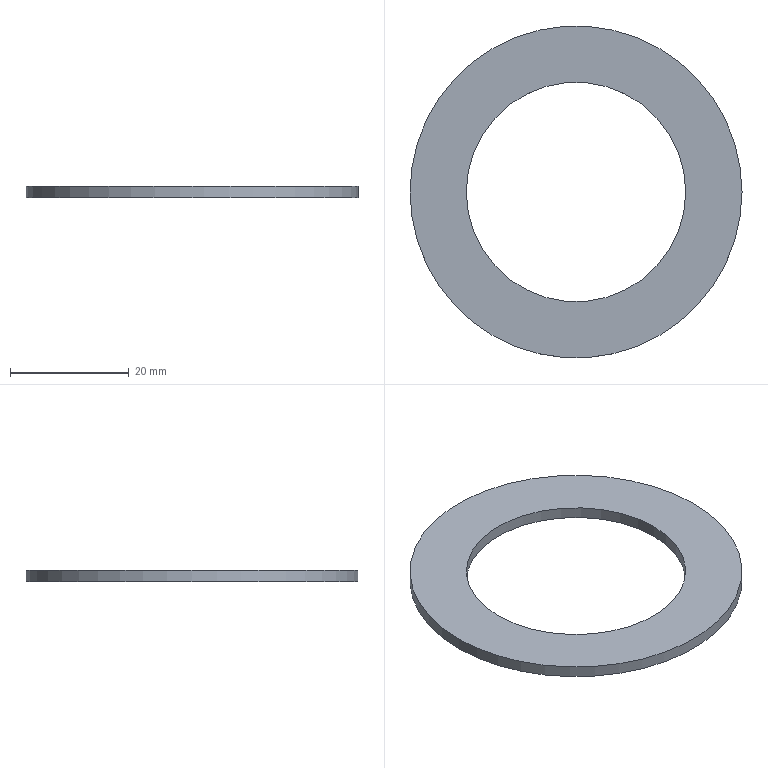Part | NX | features DATUM_CSYS 2, SKETCH 1, SWP104 1 | 1 solid | 4 faces | box 56 x 56 x 2 mm | volume 2776 mm3 | cylinder 2 | plane 2 | commonest cylinder face diameters 37 x1 56 x1
STEP:
#1=CARTESIAN_POINT('',(-18.5,0.,0.));
#2=VERTEX_POINT('',#1);
#3=CARTESIAN_POINT('',(0.,0.,0.));
#4=DIRECTION('',(0.,0.,-1.));
#5=DIRECTION('',(-1.,0.,0.));
#6=AXIS2_PLACEMENT_3D('',#3,#4,#5);
#7=CIRCLE('',#6,18.5);
#8=EDGE_CURVE('',#2,#2,#7,.T.);
#9=ORIENTED_EDGE('',*,*,#8,.T.);
#10=EDGE_LOOP('',(#9));
#11=FACE_BOUND('',#10,.T.);
#12=CARTESIAN_POINT('',(-18.5,0.,2.));
#13=VERTEX_POINT('',#12);
#14=CARTESIAN_POINT('',(0.,0.,2.));
#15=DIRECTION('',(0.,0.,-1.));
#16=DIRECTION('',(-1.,0.,0.));
#17=AXIS2_PLACEMENT_3D('',#14,#15,#16);
#18=CIRCLE('',#17,18.5);
#19=EDGE_CURVE('',#13,#13,#18,.T.);
#20=ORIENTED_EDGE('',*,*,#19,.F.);
#21=EDGE_LOOP('',(#20));
#22=FACE_BOUND('',#21,.T.);
#23=CARTESIAN_POINT('',(0.,0.,0.));
#24=DIRECTION('',(0.,0.,1.));
#25=DIRECTION('',(1.,0.,0.));
#26=AXIS2_PLACEMENT_3D('',#23,#24,#25);
#27=CYLINDRICAL_SURFACE('',#26,18.5);
#28=ADVANCED_FACE('',(#11,#22),#27,.F.);
#29=CARTESIAN_POINT('',(-28.,0.,0.));
#30=VERTEX_POINT('',#29);
#31=CARTESIAN_POINT('',(0.,0.,0.));
#32=DIRECTION('',(0.,0.,-1.));
#33=DIRECTION('',(-1.,0.,0.));
#34=AXIS2_PLACEMENT_3D('',#31,#32,#33);
#35=CIRCLE('',#34,28.);
#36=EDGE_CURVE('',#30,#30,#35,.T.);
#37=ORIENTED_EDGE('',*,*,#36,.F.);
#38=EDGE_LOOP('',(#37));
#39=FACE_BOUND('',#38,.T.);
#40=CARTESIAN_POINT('',(-28.,0.,2.));
#41=VERTEX_POINT('',#40);
#42=CARTESIAN_POINT('',(0.,0.,2.));
#43=DIRECTION('',(0.,0.,-1.));
#44=DIRECTION('',(-1.,0.,0.));
#45=AXIS2_PLACEMENT_3D('',#42,#43,#44);
#46=CIRCLE('',#45,28.);
#47=EDGE_CURVE('',#41,#41,#46,.T.);
#48=ORIENTED_EDGE('',*,*,#47,.T.);
#49=EDGE_LOOP('',(#48));
#50=FACE_BOUND('',#49,.T.);
#51=CARTESIAN_POINT('',(0.,0.,0.));
#52=DIRECTION('',(0.,0.,1.));
#53=DIRECTION('',(1.,0.,0.));
#54=AXIS2_PLACEMENT_3D('',#51,#52,#53);
#55=CYLINDRICAL_SURFACE('',#54,28.);
#56=ADVANCED_FACE('',(#39,#50),#55,.T.);
#57=ORIENTED_EDGE('',*,*,#8,.F.);
#58=EDGE_LOOP('',(#57));
#59=FACE_BOUND('',#58,.T.);
#60=ORIENTED_EDGE('',*,*,#36,.T.);
#61=EDGE_LOOP('',(#60));
#62=FACE_BOUND('',#61,.T.);
#63=CARTESIAN_POINT('',(0.,0.,0.));
#64=DIRECTION('',(0.,0.,-1.));
#65=DIRECTION('',(-1.,0.,0.));
#66=AXIS2_PLACEMENT_3D('',#63,#64,#65);
#67=PLANE('',#66);
#68=ADVANCED_FACE('',(#59,#62),#67,.T.);
#69=ORIENTED_EDGE('',*,*,#19,.T.);
#70=EDGE_LOOP('',(#69));
#71=FACE_BOUND('',#70,.T.);
#72=ORIENTED_EDGE('',*,*,#47,.F.);
#73=EDGE_LOOP('',(#72));
#74=FACE_BOUND('',#73,.T.);
#75=CARTESIAN_POINT('',(0.,0.,2.));
#76=DIRECTION('',(0.,0.,-1.));
#77=DIRECTION('',(-1.,0.,0.));
#78=AXIS2_PLACEMENT_3D('',#75,#76,#77);
#79=PLANE('',#78);
#80=ADVANCED_FACE('',(#71,#74),#79,.F.);
#81=CLOSED_SHELL('',(#28,#56,#68,#80));
#82=MANIFOLD_SOLID_BREP('',#81);
#83=(LENGTH_UNIT()NAMED_UNIT(*)SI_UNIT(.MILLI.,.METRE.));
#84=UNCERTAINTY_MEASURE_WITH_UNIT(LENGTH_MEASURE(0.00001),#83,'','');
#85=(NAMED_UNIT(*)PLANE_ANGLE_UNIT()SI_UNIT($,.RADIAN.));
#86=(NAMED_UNIT(*)SI_UNIT($,.STERADIAN.)SOLID_ANGLE_UNIT());
#87=(GEOMETRIC_REPRESENTATION_CONTEXT(3)GLOBAL_UNCERTAINTY_ASSIGNED_CONTEXT((#84))GLOBAL_UNIT_ASSIGNED_CONTEXT((#83,#85,#86))REPRESENTATION_CONTEXT('',''));
#88=ADVANCED_BREP_SHAPE_REPRESENTATION('',(#82),#87);